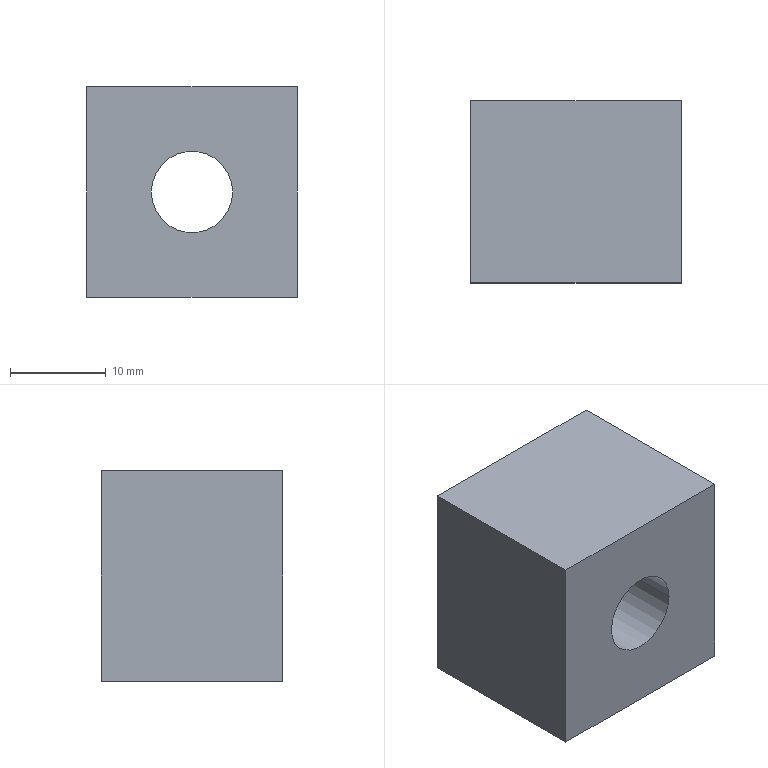Part | SolidWorks | features BaseBody 1 | 1 solid | 8 faces | box 22 x 19 x 22 mm | volume 8118 mm3 | plane 6 | cylinder 2 | commonest cylinder face diameters 8.5 x2
STEP:
#1=CARTESIAN_POINT('',(-11.,19.,-11.));
#2=VERTEX_POINT('',#1);
#3=CARTESIAN_POINT('',(-11.,0.,-11.));
#4=VERTEX_POINT('',#3);
#5=CARTESIAN_POINT('',(-11.,19.,-11.));
#6=DIRECTION('',(0.,-1.,0.));
#7=VECTOR('',#6,1000.);
#8=LINE('',#5,#7);
#9=EDGE_CURVE('',#2,#4,#8,.T.);
#10=ORIENTED_EDGE('',*,*,#9,.F.);
#11=CARTESIAN_POINT('',(11.,19.,-11.));
#12=VERTEX_POINT('',#11);
#13=CARTESIAN_POINT('',(11.,19.,-11.));
#14=DIRECTION('',(-1.,0.,0.));
#15=VECTOR('',#14,1000.);
#16=LINE('',#13,#15);
#17=EDGE_CURVE('',#12,#2,#16,.T.);
#18=ORIENTED_EDGE('',*,*,#17,.F.);
#19=CARTESIAN_POINT('',(11.,0.,-11.));
#20=VERTEX_POINT('',#19);
#21=CARTESIAN_POINT('',(11.,0.,-11.));
#22=DIRECTION('',(0.,1.,0.));
#23=VECTOR('',#22,1000.);
#24=LINE('',#21,#23);
#25=EDGE_CURVE('',#20,#12,#24,.T.);
#26=ORIENTED_EDGE('',*,*,#25,.F.);
#27=CARTESIAN_POINT('',(-11.,0.,-11.));
#28=DIRECTION('',(1.,0.,0.));
#29=VECTOR('',#28,1000.);
#30=LINE('',#27,#29);
#31=EDGE_CURVE('',#4,#20,#30,.T.);
#32=ORIENTED_EDGE('',*,*,#31,.F.);
#33=EDGE_LOOP('',(#10,#18,#26,#32));
#34=FACE_OUTER_BOUND('',#33,.T.);
#35=CARTESIAN_POINT('',(0.,0.,-11.));
#36=DIRECTION('',(0.,0.,1.));
#37=DIRECTION('',(1.,0.,0.));
#38=AXIS2_PLACEMENT_3D('',#35,#36,#37);
#39=PLANE('',#38);
#40=ADVANCED_FACE('',(#34),#39,.F.);
#41=CARTESIAN_POINT('',(11.,0.,11.));
#42=VERTEX_POINT('',#41);
#43=CARTESIAN_POINT('',(11.,0.,-11.));
#44=DIRECTION('',(0.,0.,1.));
#45=VECTOR('',#44,1000.);
#46=LINE('',#43,#45);
#47=EDGE_CURVE('',#20,#42,#46,.T.);
#48=ORIENTED_EDGE('',*,*,#47,.T.);
#49=CARTESIAN_POINT('',(-11.,0.,11.));
#50=VERTEX_POINT('',#49);
#51=CARTESIAN_POINT('',(-11.,0.,11.));
#52=DIRECTION('',(1.,0.,0.));
#53=VECTOR('',#52,1000.);
#54=LINE('',#51,#53);
#55=EDGE_CURVE('',#50,#42,#54,.T.);
#56=ORIENTED_EDGE('',*,*,#55,.F.);
#57=CARTESIAN_POINT('',(-11.,0.,-11.));
#58=DIRECTION('',(0.,0.,1.));
#59=VECTOR('',#58,1000.);
#60=LINE('',#57,#59);
#61=EDGE_CURVE('',#4,#50,#60,.T.);
#62=ORIENTED_EDGE('',*,*,#61,.F.);
#63=ORIENTED_EDGE('',*,*,#31,.T.);
#64=EDGE_LOOP('',(#48,#56,#62,#63));
#65=FACE_OUTER_BOUND('',#64,.T.);
#66=CARTESIAN_POINT('',(-4.25,0.,0.));
#67=VERTEX_POINT('',#66);
#68=CARTESIAN_POINT('',(4.25,0.,0.));
#69=VERTEX_POINT('',#68);
#70=CARTESIAN_POINT('',(0.,0.,0.));
#71=DIRECTION('',(0.,-1.,0.));
#72=DIRECTION('',(-1.,0.,0.));
#73=AXIS2_PLACEMENT_3D('',#70,#71,#72);
#74=CIRCLE('',#73,4.25);
#75=EDGE_CURVE('',#67,#69,#74,.T.);
#76=ORIENTED_EDGE('',*,*,#75,.F.);
#77=CARTESIAN_POINT('',(0.,0.,0.));
#78=DIRECTION('',(0.,-1.,0.));
#79=DIRECTION('',(1.,0.,0.));
#80=AXIS2_PLACEMENT_3D('',#77,#78,#79);
#81=CIRCLE('',#80,4.25);
#82=EDGE_CURVE('',#69,#67,#81,.T.);
#83=ORIENTED_EDGE('',*,*,#82,.F.);
#84=EDGE_LOOP('',(#76,#83));
#85=FACE_BOUND('',#84,.T.);
#86=CARTESIAN_POINT('',(-11.,0.,-11.));
#87=DIRECTION('',(0.,-1.,0.));
#88=DIRECTION('',(0.,0.,-1.));
#89=AXIS2_PLACEMENT_3D('',#86,#87,#88);
#90=PLANE('',#89);
#91=ADVANCED_FACE('',(#65,#85),#90,.T.);
#92=ORIENTED_EDGE('',*,*,#61,.T.);
#93=CARTESIAN_POINT('',(-11.,19.,11.));
#94=VERTEX_POINT('',#93);
#95=CARTESIAN_POINT('',(-11.,19.,11.));
#96=DIRECTION('',(0.,-1.,0.));
#97=VECTOR('',#96,1000.);
#98=LINE('',#95,#97);
#99=EDGE_CURVE('',#94,#50,#98,.T.);
#100=ORIENTED_EDGE('',*,*,#99,.F.);
#101=CARTESIAN_POINT('',(-11.,19.,-11.));
#102=DIRECTION('',(0.,0.,1.));
#103=VECTOR('',#102,1000.);
#104=LINE('',#101,#103);
#105=EDGE_CURVE('',#2,#94,#104,.T.);
#106=ORIENTED_EDGE('',*,*,#105,.F.);
#107=ORIENTED_EDGE('',*,*,#9,.T.);
#108=EDGE_LOOP('',(#92,#100,#106,#107));
#109=FACE_OUTER_BOUND('',#108,.T.);
#110=CARTESIAN_POINT('',(-11.,19.,-11.));
#111=DIRECTION('',(-1.,0.,0.));
#112=DIRECTION('',(0.,0.,1.));
#113=AXIS2_PLACEMENT_3D('',#110,#111,#112);
#114=PLANE('',#113);
#115=ADVANCED_FACE('',(#109),#114,.T.);
#116=ORIENTED_EDGE('',*,*,#105,.T.);
#117=CARTESIAN_POINT('',(11.,19.,11.));
#118=VERTEX_POINT('',#117);
#119=CARTESIAN_POINT('',(11.,19.,11.));
#120=DIRECTION('',(-1.,0.,0.));
#121=VECTOR('',#120,1000.);
#122=LINE('',#119,#121);
#123=EDGE_CURVE('',#118,#94,#122,.T.);
#124=ORIENTED_EDGE('',*,*,#123,.F.);
#125=CARTESIAN_POINT('',(11.,19.,-11.));
#126=DIRECTION('',(0.,0.,1.));
#127=VECTOR('',#126,1000.);
#128=LINE('',#125,#127);
#129=EDGE_CURVE('',#12,#118,#128,.T.);
#130=ORIENTED_EDGE('',*,*,#129,.F.);
#131=ORIENTED_EDGE('',*,*,#17,.T.);
#132=EDGE_LOOP('',(#116,#124,#130,#131));
#133=FACE_OUTER_BOUND('',#132,.T.);
#134=CARTESIAN_POINT('',(-4.25,19.,0.));
#135=VERTEX_POINT('',#134);
#136=CARTESIAN_POINT('',(4.25,19.,0.));
#137=VERTEX_POINT('',#136);
#138=CARTESIAN_POINT('',(0.,19.,0.));
#139=DIRECTION('',(0.,-1.,0.));
#140=DIRECTION('',(-1.,0.,0.));
#141=AXIS2_PLACEMENT_3D('',#138,#139,#140);
#142=CIRCLE('',#141,4.25);
#143=EDGE_CURVE('',#135,#137,#142,.T.);
#144=ORIENTED_EDGE('',*,*,#143,.T.);
#145=CARTESIAN_POINT('',(0.,19.,0.));
#146=DIRECTION('',(0.,-1.,0.));
#147=DIRECTION('',(1.,0.,0.));
#148=AXIS2_PLACEMENT_3D('',#145,#146,#147);
#149=CIRCLE('',#148,4.25);
#150=EDGE_CURVE('',#137,#135,#149,.T.);
#151=ORIENTED_EDGE('',*,*,#150,.T.);
#152=EDGE_LOOP('',(#144,#151));
#153=FACE_BOUND('',#152,.T.);
#154=CARTESIAN_POINT('',(11.,19.,-11.));
#155=DIRECTION('',(0.,1.,0.));
#156=DIRECTION('',(1.,0.,0.));
#157=AXIS2_PLACEMENT_3D('',#154,#155,#156);
#158=PLANE('',#157);
#159=ADVANCED_FACE('',(#133,#153),#158,.T.);
#160=ORIENTED_EDGE('',*,*,#129,.T.);
#161=CARTESIAN_POINT('',(11.,0.,11.));
#162=DIRECTION('',(0.,1.,0.));
#163=VECTOR('',#162,1000.);
#164=LINE('',#161,#163);
#165=EDGE_CURVE('',#42,#118,#164,.T.);
#166=ORIENTED_EDGE('',*,*,#165,.F.);
#167=ORIENTED_EDGE('',*,*,#47,.F.);
#168=ORIENTED_EDGE('',*,*,#25,.T.);
#169=EDGE_LOOP('',(#160,#166,#167,#168));
#170=FACE_OUTER_BOUND('',#169,.T.);
#171=CARTESIAN_POINT('',(11.,0.,-11.));
#172=DIRECTION('',(1.,0.,0.));
#173=DIRECTION('',(0.,1.,0.));
#174=AXIS2_PLACEMENT_3D('',#171,#172,#173);
#175=PLANE('',#174);
#176=ADVANCED_FACE('',(#170),#175,.T.);
#177=ORIENTED_EDGE('',*,*,#165,.T.);
#178=ORIENTED_EDGE('',*,*,#123,.T.);
#179=ORIENTED_EDGE('',*,*,#99,.T.);
#180=ORIENTED_EDGE('',*,*,#55,.T.);
#181=EDGE_LOOP('',(#177,#178,#179,#180));
#182=FACE_OUTER_BOUND('',#181,.T.);
#183=CARTESIAN_POINT('',(0.,0.,11.));
#184=DIRECTION('',(0.,0.,1.));
#185=DIRECTION('',(1.,0.,0.));
#186=AXIS2_PLACEMENT_3D('',#183,#184,#185);
#187=PLANE('',#186);
#188=ADVANCED_FACE('',(#182),#187,.T.);
#189=CARTESIAN_POINT('',(-4.25,19.,0.));
#190=DIRECTION('',(0.,-1.,0.));
#191=VECTOR('',#190,1000.);
#192=LINE('',#189,#191);
#193=EDGE_CURVE('',#135,#67,#192,.T.);
#194=ORIENTED_EDGE('',*,*,#193,.F.);
#195=ORIENTED_EDGE('',*,*,#150,.F.);
#196=CARTESIAN_POINT('',(4.25,19.,0.));
#197=DIRECTION('',(0.,-1.,0.));
#198=VECTOR('',#197,1000.);
#199=LINE('',#196,#198);
#200=EDGE_CURVE('',#137,#69,#199,.T.);
#201=ORIENTED_EDGE('',*,*,#200,.T.);
#202=ORIENTED_EDGE('',*,*,#82,.T.);
#203=EDGE_LOOP('',(#194,#195,#201,#202));
#204=FACE_OUTER_BOUND('',#203,.T.);
#205=CARTESIAN_POINT('',(0.,19.,0.));
#206=DIRECTION('',(0.,-1.,0.));
#207=DIRECTION('',(1.,0.,0.));
#208=AXIS2_PLACEMENT_3D('',#205,#206,#207);
#209=CYLINDRICAL_SURFACE('',#208,4.25);
#210=ADVANCED_FACE('',(#204),#209,.F.);
#211=ORIENTED_EDGE('',*,*,#200,.F.);
#212=ORIENTED_EDGE('',*,*,#143,.F.);
#213=ORIENTED_EDGE('',*,*,#193,.T.);
#214=ORIENTED_EDGE('',*,*,#75,.T.);
#215=EDGE_LOOP('',(#211,#212,#213,#214));
#216=FACE_OUTER_BOUND('',#215,.T.);
#217=CARTESIAN_POINT('',(0.,19.,0.));
#218=DIRECTION('',(0.,-1.,0.));
#219=DIRECTION('',(1.,0.,0.));
#220=AXIS2_PLACEMENT_3D('',#217,#218,#219);
#221=CYLINDRICAL_SURFACE('',#220,4.25);
#222=ADVANCED_FACE('',(#216),#221,.F.);
#223=CLOSED_SHELL('',(#40,#91,#115,#159,#176,#188,#210,#222));
#224=MANIFOLD_SOLID_BREP('',#223);
#225=CARTESIAN_POINT('',(0.,0.,0.));
#226=DIRECTION('',(0.,0.,1.));
#227=DIRECTION('',(1.,0.,0.));
#228=AXIS2_PLACEMENT_3D('',#225,#226,#227);
#229=(LENGTH_UNIT()NAMED_UNIT(*)SI_UNIT(.MILLI.,.METRE.));
#230=UNCERTAINTY_MEASURE_WITH_UNIT(LENGTH_MEASURE(0.00001),#229,'','');
#231=(NAMED_UNIT(*)PLANE_ANGLE_UNIT()SI_UNIT($,.RADIAN.));
#232=(NAMED_UNIT(*)SI_UNIT($,.STERADIAN.)SOLID_ANGLE_UNIT());
#233=(GEOMETRIC_REPRESENTATION_CONTEXT(3)GLOBAL_UNCERTAINTY_ASSIGNED_CONTEXT((#230))GLOBAL_UNIT_ASSIGNED_CONTEXT((#229,#231,#232))REPRESENTATION_CONTEXT('',''));
#234=ADVANCED_BREP_SHAPE_REPRESENTATION('',(#224,#228),#233);